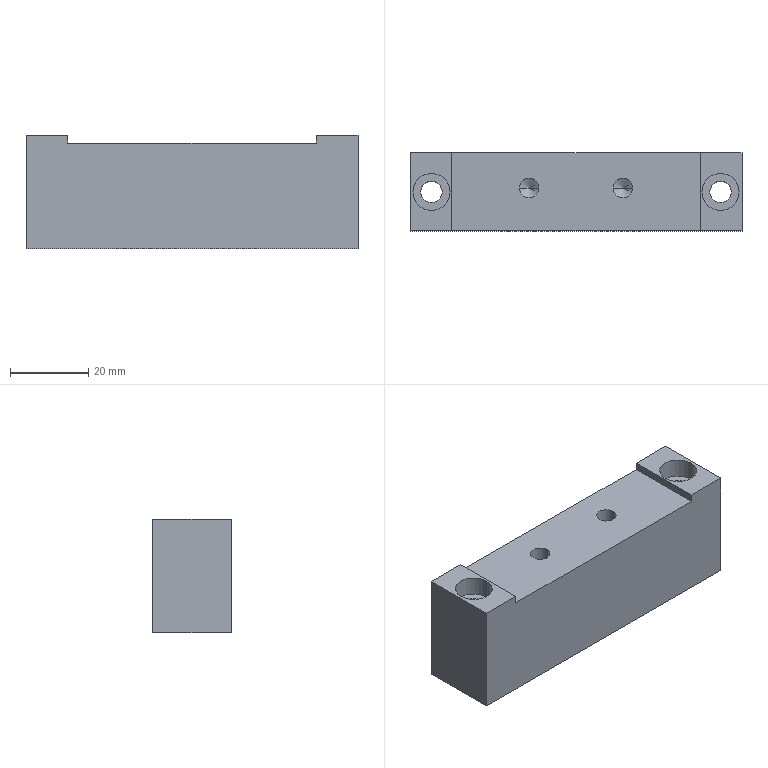Part | STEP file | 11-FG-E01211 | 1 solid | 28 faces | box 85 x 20 x 29 mm | volume 44302 mm3 | cylinder 12 | plane 12 | cone 4 | commonest cylinder face diameters 5 x4 5.5 x4 9.5 x4
STEP:
#1=CARTESIAN_POINT('',(-14.5,1.,12.));
#2=VERTEX_POINT('',#1);
#3=CARTESIAN_POINT('',(-9.5,1.,12.));
#4=VERTEX_POINT('',#3);
#5=CARTESIAN_POINT('',(-12.,1.,12.));
#6=DIRECTION('',(0.,0.,1.));
#7=DIRECTION('',(1.,0.,0.));
#8=AXIS2_PLACEMENT_3D('',#5,#6,#7);
#9=CIRCLE('',#8,2.5);
#10=EDGE_CURVE('',#2,#4,#9,.T.);
#11=ORIENTED_EDGE('',*,*,#10,.F.);
#12=CARTESIAN_POINT('',(-14.5,1.,27.));
#13=VERTEX_POINT('',#12);
#14=CARTESIAN_POINT('',(-14.5,1.,27.));
#15=DIRECTION('',(0.,0.,1.));
#16=VECTOR('',#15,1000.);
#17=LINE('',#14,#16);
#18=EDGE_CURVE('',#2,#13,#17,.T.);
#19=ORIENTED_EDGE('',*,*,#18,.T.);
#20=CARTESIAN_POINT('',(-9.5,1.,27.));
#21=VERTEX_POINT('',#20);
#22=CARTESIAN_POINT('',(-12.,1.,27.));
#23=DIRECTION('',(0.,0.,1.));
#24=DIRECTION('',(1.,0.,0.));
#25=AXIS2_PLACEMENT_3D('',#22,#23,#24);
#26=CIRCLE('',#25,2.5);
#27=EDGE_CURVE('',#13,#21,#26,.T.);
#28=ORIENTED_EDGE('',*,*,#27,.T.);
#29=CARTESIAN_POINT('',(-9.5,1.,27.));
#30=DIRECTION('',(0.,0.,1.));
#31=VECTOR('',#30,1000.);
#32=LINE('',#29,#31);
#33=EDGE_CURVE('',#4,#21,#32,.T.);
#34=ORIENTED_EDGE('',*,*,#33,.F.);
#35=EDGE_LOOP('',(#11,#19,#28,#34));
#36=FACE_OUTER_BOUND('',#35,.T.);
#37=CARTESIAN_POINT('',(-12.,1.,27.));
#38=DIRECTION('',(0.,0.,1.));
#39=DIRECTION('',(1.,0.,0.));
#40=AXIS2_PLACEMENT_3D('',#37,#38,#39);
#41=CYLINDRICAL_SURFACE('',#40,2.5);
#42=ADVANCED_FACE('',(#36),#41,.F.);
#43=CARTESIAN_POINT('',(-12.,1.,10.498));
#44=VERTEX_POINT('',#43);
#45=CARTESIAN_POINT('',(-9.5,1.,12.));
#46=DIRECTION('',(0.8572,0.,0.515));
#47=VECTOR('',#46,1000.);
#48=LINE('',#45,#47);
#49=EDGE_CURVE('',#44,#4,#48,.T.);
#50=ORIENTED_EDGE('',*,*,#49,.F.);
#51=CARTESIAN_POINT('',(-14.5,1.,12.));
#52=DIRECTION('',(-0.8572,0.,0.515));
#53=VECTOR('',#52,1000.);
#54=LINE('',#51,#53);
#55=EDGE_CURVE('',#44,#2,#54,.T.);
#56=ORIENTED_EDGE('',*,*,#55,.T.);
#57=ORIENTED_EDGE('',*,*,#10,.T.);
#58=EDGE_LOOP('',(#50,#56,#57));
#59=FACE_OUTER_BOUND('',#58,.T.);
#60=CARTESIAN_POINT('',(-12.,1.,12.));
#61=DIRECTION('',(0.,0.,1.));
#62=DIRECTION('',(1.,0.,0.));
#63=AXIS2_PLACEMENT_3D('',#60,#61,#62);
#64=CONICAL_SURFACE('',#63,2.5,1.03);
#65=ADVANCED_FACE('',(#59),#64,.F.);
#66=CARTESIAN_POINT('',(9.5,1.,12.));
#67=VERTEX_POINT('',#66);
#68=CARTESIAN_POINT('',(14.5,1.,12.));
#69=VERTEX_POINT('',#68);
#70=CARTESIAN_POINT('',(12.,1.,12.));
#71=DIRECTION('',(0.,0.,1.));
#72=DIRECTION('',(1.,0.,0.));
#73=AXIS2_PLACEMENT_3D('',#70,#71,#72);
#74=CIRCLE('',#73,2.5);
#75=EDGE_CURVE('',#67,#69,#74,.T.);
#76=ORIENTED_EDGE('',*,*,#75,.F.);
#77=CARTESIAN_POINT('',(9.5,1.,27.));
#78=VERTEX_POINT('',#77);
#79=CARTESIAN_POINT('',(9.5,1.,27.));
#80=DIRECTION('',(0.,0.,1.));
#81=VECTOR('',#80,1000.);
#82=LINE('',#79,#81);
#83=EDGE_CURVE('',#67,#78,#82,.T.);
#84=ORIENTED_EDGE('',*,*,#83,.T.);
#85=CARTESIAN_POINT('',(14.5,1.,27.));
#86=VERTEX_POINT('',#85);
#87=CARTESIAN_POINT('',(12.,1.,27.));
#88=DIRECTION('',(0.,0.,1.));
#89=DIRECTION('',(1.,0.,0.));
#90=AXIS2_PLACEMENT_3D('',#87,#88,#89);
#91=CIRCLE('',#90,2.5);
#92=EDGE_CURVE('',#78,#86,#91,.T.);
#93=ORIENTED_EDGE('',*,*,#92,.T.);
#94=CARTESIAN_POINT('',(14.5,1.,27.));
#95=DIRECTION('',(0.,0.,1.));
#96=VECTOR('',#95,1000.);
#97=LINE('',#94,#96);
#98=EDGE_CURVE('',#69,#86,#97,.T.);
#99=ORIENTED_EDGE('',*,*,#98,.F.);
#100=EDGE_LOOP('',(#76,#84,#93,#99));
#101=FACE_OUTER_BOUND('',#100,.T.);
#102=CARTESIAN_POINT('',(12.,1.,27.));
#103=DIRECTION('',(0.,0.,1.));
#104=DIRECTION('',(1.,0.,0.));
#105=AXIS2_PLACEMENT_3D('',#102,#103,#104);
#106=CYLINDRICAL_SURFACE('',#105,2.5);
#107=ADVANCED_FACE('',(#101),#106,.F.);
#108=CARTESIAN_POINT('',(12.,1.,10.498));
#109=VERTEX_POINT('',#108);
#110=CARTESIAN_POINT('',(14.5,1.,12.));
#111=DIRECTION('',(0.8572,0.,0.515));
#112=VECTOR('',#111,1000.);
#113=LINE('',#110,#112);
#114=EDGE_CURVE('',#109,#69,#113,.T.);
#115=ORIENTED_EDGE('',*,*,#114,.F.);
#116=CARTESIAN_POINT('',(9.5,1.,12.));
#117=DIRECTION('',(-0.8572,0.,0.515));
#118=VECTOR('',#117,1000.);
#119=LINE('',#116,#118);
#120=EDGE_CURVE('',#109,#67,#119,.T.);
#121=ORIENTED_EDGE('',*,*,#120,.T.);
#122=ORIENTED_EDGE('',*,*,#75,.T.);
#123=EDGE_LOOP('',(#115,#121,#122));
#124=FACE_OUTER_BOUND('',#123,.T.);
#125=CARTESIAN_POINT('',(12.,1.,12.));
#126=DIRECTION('',(0.,0.,1.));
#127=DIRECTION('',(1.,0.,0.));
#128=AXIS2_PLACEMENT_3D('',#125,#126,#127);
#129=CONICAL_SURFACE('',#128,2.5,1.03);
#130=ADVANCED_FACE('',(#124),#129,.F.);
#131=CARTESIAN_POINT('',(32.25,0.,24.));
#132=VERTEX_POINT('',#131);
#133=CARTESIAN_POINT('',(41.75,0.,24.));
#134=VERTEX_POINT('',#133);
#135=CARTESIAN_POINT('',(37.,0.,24.));
#136=DIRECTION('',(0.,0.,1.));
#137=DIRECTION('',(1.,0.,0.));
#138=AXIS2_PLACEMENT_3D('',#135,#136,#137);
#139=CIRCLE('',#138,4.75);
#140=EDGE_CURVE('',#132,#134,#139,.T.);
#141=ORIENTED_EDGE('',*,*,#140,.F.);
#142=CARTESIAN_POINT('',(32.25,0.,29.));
#143=VERTEX_POINT('',#142);
#144=CARTESIAN_POINT('',(32.25,0.,29.));
#145=DIRECTION('',(0.,0.,1.));
#146=VECTOR('',#145,1000.);
#147=LINE('',#144,#146);
#148=EDGE_CURVE('',#132,#143,#147,.T.);
#149=ORIENTED_EDGE('',*,*,#148,.T.);
#150=CARTESIAN_POINT('',(41.75,0.,29.));
#151=VERTEX_POINT('',#150);
#152=CARTESIAN_POINT('',(37.,0.,29.));
#153=DIRECTION('',(0.,0.,1.));
#154=DIRECTION('',(1.,0.,0.));
#155=AXIS2_PLACEMENT_3D('',#152,#153,#154);
#156=CIRCLE('',#155,4.75);
#157=EDGE_CURVE('',#143,#151,#156,.T.);
#158=ORIENTED_EDGE('',*,*,#157,.T.);
#159=CARTESIAN_POINT('',(41.75,0.,29.));
#160=DIRECTION('',(0.,0.,1.));
#161=VECTOR('',#160,1000.);
#162=LINE('',#159,#161);
#163=EDGE_CURVE('',#134,#151,#162,.T.);
#164=ORIENTED_EDGE('',*,*,#163,.F.);
#165=EDGE_LOOP('',(#141,#149,#158,#164));
#166=FACE_OUTER_BOUND('',#165,.T.);
#167=CARTESIAN_POINT('',(37.,0.,29.));
#168=DIRECTION('',(0.,0.,1.));
#169=DIRECTION('',(1.,0.,0.));
#170=AXIS2_PLACEMENT_3D('',#167,#168,#169);
#171=CYLINDRICAL_SURFACE('',#170,4.75);
#172=ADVANCED_FACE('',(#166),#171,.F.);
#173=CARTESIAN_POINT('',(34.25,0.,0.));
#174=VERTEX_POINT('',#173);
#175=CARTESIAN_POINT('',(39.75,0.,0.));
#176=VERTEX_POINT('',#175);
#177=CARTESIAN_POINT('',(37.,0.,0.));
#178=DIRECTION('',(0.,0.,1.));
#179=DIRECTION('',(1.,0.,0.));
#180=AXIS2_PLACEMENT_3D('',#177,#178,#179);
#181=CIRCLE('',#180,2.75);
#182=EDGE_CURVE('',#174,#176,#181,.T.);
#183=ORIENTED_EDGE('',*,*,#182,.F.);
#184=CARTESIAN_POINT('',(34.25,0.,24.));
#185=VERTEX_POINT('',#184);
#186=CARTESIAN_POINT('',(34.25,0.,29.));
#187=DIRECTION('',(0.,0.,1.));
#188=VECTOR('',#187,1000.);
#189=LINE('',#186,#188);
#190=EDGE_CURVE('',#174,#185,#189,.T.);
#191=ORIENTED_EDGE('',*,*,#190,.T.);
#192=CARTESIAN_POINT('',(39.75,0.,24.));
#193=VERTEX_POINT('',#192);
#194=CARTESIAN_POINT('',(37.,0.,24.));
#195=DIRECTION('',(0.,0.,1.));
#196=DIRECTION('',(1.,0.,0.));
#197=AXIS2_PLACEMENT_3D('',#194,#195,#196);
#198=CIRCLE('',#197,2.75);
#199=EDGE_CURVE('',#185,#193,#198,.T.);
#200=ORIENTED_EDGE('',*,*,#199,.T.);
#201=CARTESIAN_POINT('',(39.75,0.,29.));
#202=DIRECTION('',(0.,0.,1.));
#203=VECTOR('',#202,1000.);
#204=LINE('',#201,#203);
#205=EDGE_CURVE('',#176,#193,#204,.T.);
#206=ORIENTED_EDGE('',*,*,#205,.F.);
#207=EDGE_LOOP('',(#183,#191,#200,#206));
#208=FACE_OUTER_BOUND('',#207,.T.);
#209=CARTESIAN_POINT('',(37.,0.,29.));
#210=DIRECTION('',(0.,0.,1.));
#211=DIRECTION('',(1.,0.,0.));
#212=AXIS2_PLACEMENT_3D('',#209,#210,#211);
#213=CYLINDRICAL_SURFACE('',#212,2.75);
#214=ADVANCED_FACE('',(#208),#213,.F.);
#215=CARTESIAN_POINT('',(-41.75,0.,24.));
#216=VERTEX_POINT('',#215);
#217=CARTESIAN_POINT('',(-32.25,0.,24.));
#218=VERTEX_POINT('',#217);
#219=CARTESIAN_POINT('',(-37.,0.,24.));
#220=DIRECTION('',(0.,0.,1.));
#221=DIRECTION('',(1.,0.,0.));
#222=AXIS2_PLACEMENT_3D('',#219,#220,#221);
#223=CIRCLE('',#222,4.75);
#224=EDGE_CURVE('',#216,#218,#223,.T.);
#225=ORIENTED_EDGE('',*,*,#224,.F.);
#226=CARTESIAN_POINT('',(-41.75,0.,29.));
#227=VERTEX_POINT('',#226);
#228=CARTESIAN_POINT('',(-41.75,0.,29.));
#229=DIRECTION('',(0.,0.,1.));
#230=VECTOR('',#229,1000.);
#231=LINE('',#228,#230);
#232=EDGE_CURVE('',#216,#227,#231,.T.);
#233=ORIENTED_EDGE('',*,*,#232,.T.);
#234=CARTESIAN_POINT('',(-32.25,0.,29.));
#235=VERTEX_POINT('',#234);
#236=CARTESIAN_POINT('',(-37.,0.,29.));
#237=DIRECTION('',(0.,0.,1.));
#238=DIRECTION('',(1.,0.,0.));
#239=AXIS2_PLACEMENT_3D('',#236,#237,#238);
#240=CIRCLE('',#239,4.75);
#241=EDGE_CURVE('',#227,#235,#240,.T.);
#242=ORIENTED_EDGE('',*,*,#241,.T.);
#243=CARTESIAN_POINT('',(-32.25,0.,29.));
#244=DIRECTION('',(0.,0.,1.));
#245=VECTOR('',#244,1000.);
#246=LINE('',#243,#245);
#247=EDGE_CURVE('',#218,#235,#246,.T.);
#248=ORIENTED_EDGE('',*,*,#247,.F.);
#249=EDGE_LOOP('',(#225,#233,#242,#248));
#250=FACE_OUTER_BOUND('',#249,.T.);
#251=CARTESIAN_POINT('',(-37.,0.,29.));
#252=DIRECTION('',(0.,0.,1.));
#253=DIRECTION('',(1.,0.,0.));
#254=AXIS2_PLACEMENT_3D('',#251,#252,#253);
#255=CYLINDRICAL_SURFACE('',#254,4.75);
#256=ADVANCED_FACE('',(#250),#255,.F.);
#257=CARTESIAN_POINT('',(-39.75,0.,0.));
#258=VERTEX_POINT('',#257);
#259=CARTESIAN_POINT('',(-34.25,0.,0.));
#260=VERTEX_POINT('',#259);
#261=CARTESIAN_POINT('',(-37.,0.,0.));
#262=DIRECTION('',(0.,0.,1.));
#263=DIRECTION('',(1.,0.,0.));
#264=AXIS2_PLACEMENT_3D('',#261,#262,#263);
#265=CIRCLE('',#264,2.75);
#266=EDGE_CURVE('',#258,#260,#265,.T.);
#267=ORIENTED_EDGE('',*,*,#266,.F.);
#268=CARTESIAN_POINT('',(-39.75,0.,24.));
#269=VERTEX_POINT('',#268);
#270=CARTESIAN_POINT('',(-39.75,0.,29.));
#271=DIRECTION('',(0.,0.,1.));
#272=VECTOR('',#271,1000.);
#273=LINE('',#270,#272);
#274=EDGE_CURVE('',#258,#269,#273,.T.);
#275=ORIENTED_EDGE('',*,*,#274,.T.);
#276=CARTESIAN_POINT('',(-34.25,0.,24.));
#277=VERTEX_POINT('',#276);
#278=CARTESIAN_POINT('',(-37.,0.,24.));
#279=DIRECTION('',(0.,0.,1.));
#280=DIRECTION('',(1.,0.,0.));
#281=AXIS2_PLACEMENT_3D('',#278,#279,#280);
#282=CIRCLE('',#281,2.75);
#283=EDGE_CURVE('',#269,#277,#282,.T.);
#284=ORIENTED_EDGE('',*,*,#283,.T.);
#285=CARTESIAN_POINT('',(-34.25,0.,29.));
#286=DIRECTION('',(0.,0.,1.));
#287=VECTOR('',#286,1000.);
#288=LINE('',#285,#287);
#289=EDGE_CURVE('',#260,#277,#288,.T.);
#290=ORIENTED_EDGE('',*,*,#289,.F.);
#291=EDGE_LOOP('',(#267,#275,#284,#290));
#292=FACE_OUTER_BOUND('',#291,.T.);
#293=CARTESIAN_POINT('',(-37.,0.,29.));
#294=DIRECTION('',(0.,0.,1.));
#295=DIRECTION('',(1.,0.,0.));
#296=AXIS2_PLACEMENT_3D('',#293,#294,#295);
#297=CYLINDRICAL_SURFACE('',#296,2.75);
#298=ADVANCED_FACE('',(#292),#297,.F.);
#299=CARTESIAN_POINT('',(-37.,0.,29.));
#300=DIRECTION('',(0.,0.,1.));
#301=DIRECTION('',(1.,0.,0.));
#302=AXIS2_PLACEMENT_3D('',#299,#300,#301);
#303=CIRCLE('',#302,4.75);
#304=EDGE_CURVE('',#235,#227,#303,.T.);
#305=ORIENTED_EDGE('',*,*,#304,.F.);
#306=ORIENTED_EDGE('',*,*,#241,.F.);
#307=EDGE_LOOP('',(#305,#306));
#308=FACE_BOUND('',#307,.T.);
#309=CARTESIAN_POINT('',(-31.75,-10.,29.));
#310=VERTEX_POINT('',#309);
#311=CARTESIAN_POINT('',(-31.75,10.,29.));
#312=VERTEX_POINT('',#311);
#313=CARTESIAN_POINT('',(-31.75,-10.,29.));
#314=DIRECTION('',(0.,1.,0.));
#315=VECTOR('',#314,1000.);
#316=LINE('',#313,#315);
#317=EDGE_CURVE('',#310,#312,#316,.T.);
#318=ORIENTED_EDGE('',*,*,#317,.T.);
#319=CARTESIAN_POINT('',(-42.5,10.,29.));
#320=VERTEX_POINT('',#319);
#321=CARTESIAN_POINT('',(-42.5,10.,29.));
#322=DIRECTION('',(-1.,0.,0.));
#323=VECTOR('',#322,1000.);
#324=LINE('',#321,#323);
#325=EDGE_CURVE('',#312,#320,#324,.T.);
#326=ORIENTED_EDGE('',*,*,#325,.T.);
#327=CARTESIAN_POINT('',(-42.5,-10.,29.));
#328=VERTEX_POINT('',#327);
#329=CARTESIAN_POINT('',(-42.5,10.,29.));
#330=DIRECTION('',(0.,-1.,0.));
#331=VECTOR('',#330,1000.);
#332=LINE('',#329,#331);
#333=EDGE_CURVE('',#320,#328,#332,.T.);
#334=ORIENTED_EDGE('',*,*,#333,.T.);
#335=CARTESIAN_POINT('',(-42.5,-10.,29.));
#336=DIRECTION('',(1.,0.,0.));
#337=VECTOR('',#336,1000.);
#338=LINE('',#335,#337);
#339=EDGE_CURVE('',#328,#310,#338,.T.);
#340=ORIENTED_EDGE('',*,*,#339,.T.);
#341=EDGE_LOOP('',(#318,#326,#334,#340));
#342=FACE_OUTER_BOUND('',#341,.T.);
#343=CARTESIAN_POINT('',(42.5,-10.,29.));
#344=DIRECTION('',(0.,0.,1.));
#345=DIRECTION('',(1.,0.,0.));
#346=AXIS2_PLACEMENT_3D('',#343,#344,#345);
#347=PLANE('',#346);
#348=ADVANCED_FACE('',(#308,#342),#347,.T.);
#349=CARTESIAN_POINT('',(42.5,-10.,0.));
#350=VERTEX_POINT('',#349);
#351=CARTESIAN_POINT('',(42.5,10.,0.));
#352=VERTEX_POINT('',#351);
#353=CARTESIAN_POINT('',(42.5,10.,0.));
#354=DIRECTION('',(0.,1.,0.));
#355=VECTOR('',#354,1000.);
#356=LINE('',#353,#355);
#357=EDGE_CURVE('',#350,#352,#356,.T.);
#358=ORIENTED_EDGE('',*,*,#357,.T.);
#359=CARTESIAN_POINT('',(42.5,10.,29.));
#360=VERTEX_POINT('',#359);
#361=CARTESIAN_POINT('',(42.5,10.,29.));
#362=DIRECTION('',(0.,0.,-1.));
#363=VECTOR('',#362,1000.);
#364=LINE('',#361,#363);
#365=EDGE_CURVE('',#360,#352,#364,.T.);
#366=ORIENTED_EDGE('',*,*,#365,.F.);
#367=CARTESIAN_POINT('',(42.5,-10.,29.));
#368=VERTEX_POINT('',#367);
#369=CARTESIAN_POINT('',(42.5,10.,29.));
#370=DIRECTION('',(0.,1.,0.));
#371=VECTOR('',#370,1000.);
#372=LINE('',#369,#371);
#373=EDGE_CURVE('',#368,#360,#372,.T.);
#374=ORIENTED_EDGE('',*,*,#373,.F.);
#375=CARTESIAN_POINT('',(42.5,-10.,29.));
#376=DIRECTION('',(0.,0.,-1.));
#377=VECTOR('',#376,1000.);
#378=LINE('',#375,#377);
#379=EDGE_CURVE('',#368,#350,#378,.T.);
#380=ORIENTED_EDGE('',*,*,#379,.T.);
#381=EDGE_LOOP('',(#358,#366,#374,#380));
#382=FACE_OUTER_BOUND('',#381,.T.);
#383=CARTESIAN_POINT('',(42.5,10.,29.));
#384=DIRECTION('',(-1.,0.,0.));
#385=DIRECTION('',(0.,0.,1.));
#386=AXIS2_PLACEMENT_3D('',#383,#384,#385);
#387=PLANE('',#386);
#388=ADVANCED_FACE('',(#382),#387,.F.);
#389=ORIENTED_EDGE('',*,*,#325,.F.);
#390=CARTESIAN_POINT('',(-31.75,10.,27.));
#391=VERTEX_POINT('',#390);
#392=CARTESIAN_POINT('',(-31.75,10.,27.));
#393=DIRECTION('',(0.,0.,1.));
#394=VECTOR('',#393,1000.);
#395=LINE('',#392,#394);
#396=EDGE_CURVE('',#391,#312,#395,.T.);
#397=ORIENTED_EDGE('',*,*,#396,.F.);
#398=CARTESIAN_POINT('',(31.75,10.,27.));
#399=VERTEX_POINT('',#398);
#400=CARTESIAN_POINT('',(-31.75,10.,27.));
#401=DIRECTION('',(-1.,0.,0.));
#402=VECTOR('',#401,1000.);
#403=LINE('',#400,#402);
#404=EDGE_CURVE('',#399,#391,#403,.T.);
#405=ORIENTED_EDGE('',*,*,#404,.F.);
#406=CARTESIAN_POINT('',(31.75,10.,29.));
#407=VERTEX_POINT('',#406);
#408=CARTESIAN_POINT('',(31.75,10.,27.));
#409=DIRECTION('',(0.,0.,-1.));
#410=VECTOR('',#409,1000.);
#411=LINE('',#408,#410);
#412=EDGE_CURVE('',#407,#399,#411,.T.);
#413=ORIENTED_EDGE('',*,*,#412,.F.);
#414=CARTESIAN_POINT('',(-42.5,10.,29.));
#415=DIRECTION('',(-1.,0.,0.));
#416=VECTOR('',#415,1000.);
#417=LINE('',#414,#416);
#418=EDGE_CURVE('',#360,#407,#417,.T.);
#419=ORIENTED_EDGE('',*,*,#418,.F.);
#420=ORIENTED_EDGE('',*,*,#365,.T.);
#421=CARTESIAN_POINT('',(-42.5,10.,0.));
#422=VERTEX_POINT('',#421);
#423=CARTESIAN_POINT('',(-42.5,10.,0.));
#424=DIRECTION('',(-1.,0.,0.));
#425=VECTOR('',#424,1000.);
#426=LINE('',#423,#425);
#427=EDGE_CURVE('',#352,#422,#426,.T.);
#428=ORIENTED_EDGE('',*,*,#427,.T.);
#429=CARTESIAN_POINT('',(-42.5,10.,29.));
#430=DIRECTION('',(0.,0.,-1.));
#431=VECTOR('',#430,1000.);
#432=LINE('',#429,#431);
#433=EDGE_CURVE('',#320,#422,#432,.T.);
#434=ORIENTED_EDGE('',*,*,#433,.F.);
#435=EDGE_LOOP('',(#389,#397,#405,#413,#419,#420,#428,#434));
#436=FACE_OUTER_BOUND('',#435,.T.);
#437=CARTESIAN_POINT('',(-42.5,10.,29.));
#438=DIRECTION('',(0.,-1.,0.));
#439=DIRECTION('',(0.,0.,-1.));
#440=AXIS2_PLACEMENT_3D('',#437,#438,#439);
#441=PLANE('',#440);
#442=ADVANCED_FACE('',(#436),#441,.F.);
#443=CARTESIAN_POINT('',(-42.5,-10.,0.));
#444=VERTEX_POINT('',#443);
#445=CARTESIAN_POINT('',(-42.5,10.,0.));
#446=DIRECTION('',(0.,-1.,0.));
#447=VECTOR('',#446,1000.);
#448=LINE('',#445,#447);
#449=EDGE_CURVE('',#422,#444,#448,.T.);
#450=ORIENTED_EDGE('',*,*,#449,.T.);
#451=CARTESIAN_POINT('',(-42.5,-10.,29.));
#452=DIRECTION('',(0.,0.,-1.));
#453=VECTOR('',#452,1000.);
#454=LINE('',#451,#453);
#455=EDGE_CURVE('',#328,#444,#454,.T.);
#456=ORIENTED_EDGE('',*,*,#455,.F.);
#457=ORIENTED_EDGE('',*,*,#333,.F.);
#458=ORIENTED_EDGE('',*,*,#433,.T.);
#459=EDGE_LOOP('',(#450,#456,#457,#458));
#460=FACE_OUTER_BOUND('',#459,.T.);
#461=CARTESIAN_POINT('',(-42.5,10.,29.));
#462=DIRECTION('',(1.,0.,0.));
#463=DIRECTION('',(0.,0.,-1.));
#464=AXIS2_PLACEMENT_3D('',#461,#462,#463);
#465=PLANE('',#464);
#466=ADVANCED_FACE('',(#460),#465,.F.);
#467=CARTESIAN_POINT('',(31.75,-10.,27.));
#468=VERTEX_POINT('',#467);
#469=CARTESIAN_POINT('',(-31.75,-10.,27.));
#470=VERTEX_POINT('',#469);
#471=CARTESIAN_POINT('',(-31.75,-10.,27.));
#472=DIRECTION('',(-1.,0.,0.));
#473=VECTOR('',#472,1000.);
#474=LINE('',#471,#473);
#475=EDGE_CURVE('',#468,#470,#474,.T.);
#476=ORIENTED_EDGE('',*,*,#475,.T.);
#477=CARTESIAN_POINT('',(-31.75,-10.,27.));
#478=DIRECTION('',(0.,0.,1.));
#479=VECTOR('',#478,1000.);
#480=LINE('',#477,#479);
#481=EDGE_CURVE('',#470,#310,#480,.T.);
#482=ORIENTED_EDGE('',*,*,#481,.T.);
#483=ORIENTED_EDGE('',*,*,#339,.F.);
#484=ORIENTED_EDGE('',*,*,#455,.T.);
#485=CARTESIAN_POINT('',(-42.5,-10.,0.));
#486=DIRECTION('',(1.,0.,0.));
#487=VECTOR('',#486,1000.);
#488=LINE('',#485,#487);
#489=EDGE_CURVE('',#444,#350,#488,.T.);
#490=ORIENTED_EDGE('',*,*,#489,.T.);
#491=ORIENTED_EDGE('',*,*,#379,.F.);
#492=CARTESIAN_POINT('',(31.75,-10.,29.));
#493=VERTEX_POINT('',#492);
#494=CARTESIAN_POINT('',(-42.5,-10.,29.));
#495=DIRECTION('',(1.,0.,0.));
#496=VECTOR('',#495,1000.);
#497=LINE('',#494,#496);
#498=EDGE_CURVE('',#493,#368,#497,.T.);
#499=ORIENTED_EDGE('',*,*,#498,.F.);
#500=CARTESIAN_POINT('',(31.75,-10.,27.));
#501=DIRECTION('',(0.,0.,-1.));
#502=VECTOR('',#501,1000.);
#503=LINE('',#500,#502);
#504=EDGE_CURVE('',#493,#468,#503,.T.);
#505=ORIENTED_EDGE('',*,*,#504,.T.);
#506=EDGE_LOOP('',(#476,#482,#483,#484,#490,#491,#499,#505));
#507=FACE_OUTER_BOUND('',#506,.T.);
#508=CARTESIAN_POINT('',(-42.5,-10.,29.));
#509=DIRECTION('',(0.,1.,0.));
#510=DIRECTION('',(0.,0.,1.));
#511=AXIS2_PLACEMENT_3D('',#508,#509,#510);
#512=PLANE('',#511);
#513=ADVANCED_FACE('',(#507),#512,.F.);
#514=CARTESIAN_POINT('',(37.,0.,29.));
#515=DIRECTION('',(0.,0.,1.));
#516=DIRECTION('',(1.,0.,0.));
#517=AXIS2_PLACEMENT_3D('',#514,#515,#516);
#518=CIRCLE('',#517,4.75);
#519=EDGE_CURVE('',#151,#143,#518,.T.);
#520=ORIENTED_EDGE('',*,*,#519,.F.);
#521=ORIENTED_EDGE('',*,*,#157,.F.);
#522=EDGE_LOOP('',(#520,#521));
#523=FACE_BOUND('',#522,.T.);
#524=CARTESIAN_POINT('',(31.75,-10.,29.));
#525=DIRECTION('',(0.,1.,0.));
#526=VECTOR('',#525,1000.);
#527=LINE('',#524,#526);
#528=EDGE_CURVE('',#493,#407,#527,.T.);
#529=ORIENTED_EDGE('',*,*,#528,.F.);
#530=ORIENTED_EDGE('',*,*,#498,.T.);
#531=ORIENTED_EDGE('',*,*,#373,.T.);
#532=ORIENTED_EDGE('',*,*,#418,.T.);
#533=EDGE_LOOP('',(#529,#530,#531,#532));
#534=FACE_OUTER_BOUND('',#533,.T.);
#535=CARTESIAN_POINT('',(42.5,-10.,29.));
#536=DIRECTION('',(0.,0.,1.));
#537=DIRECTION('',(1.,0.,0.));
#538=AXIS2_PLACEMENT_3D('',#535,#536,#537);
#539=PLANE('',#538);
#540=ADVANCED_FACE('',(#523,#534),#539,.T.);
#541=CARTESIAN_POINT('',(37.,0.,0.));
#542=DIRECTION('',(0.,0.,1.));
#543=DIRECTION('',(1.,0.,0.));
#544=AXIS2_PLACEMENT_3D('',#541,#542,#543);
#545=CIRCLE('',#544,2.75);
#546=EDGE_CURVE('',#176,#174,#545,.T.);
#547=ORIENTED_EDGE('',*,*,#546,.T.);
#548=ORIENTED_EDGE('',*,*,#182,.T.);
#549=EDGE_LOOP('',(#547,#548));
#550=FACE_BOUND('',#549,.T.);
#551=CARTESIAN_POINT('',(-37.,0.,0.));
#552=DIRECTION('',(0.,0.,1.));
#553=DIRECTION('',(1.,0.,0.));
#554=AXIS2_PLACEMENT_3D('',#551,#552,#553);
#555=CIRCLE('',#554,2.75);
#556=EDGE_CURVE('',#260,#258,#555,.T.);
#557=ORIENTED_EDGE('',*,*,#556,.T.);
#558=ORIENTED_EDGE('',*,*,#266,.T.);
#559=EDGE_LOOP('',(#557,#558));
#560=FACE_BOUND('',#559,.T.);
#561=ORIENTED_EDGE('',*,*,#357,.F.);
#562=ORIENTED_EDGE('',*,*,#489,.F.);
#563=ORIENTED_EDGE('',*,*,#449,.F.);
#564=ORIENTED_EDGE('',*,*,#427,.F.);
#565=EDGE_LOOP('',(#561,#562,#563,#564));
#566=FACE_OUTER_BOUND('',#565,.T.);
#567=CARTESIAN_POINT('',(42.5,-10.,0.));
#568=DIRECTION('',(0.,0.,1.));
#569=DIRECTION('',(1.,0.,0.));
#570=AXIS2_PLACEMENT_3D('',#567,#568,#569);
#571=PLANE('',#570);
#572=ADVANCED_FACE('',(#550,#560,#566),#571,.F.);
#573=ORIENTED_EDGE('',*,*,#396,.T.);
#574=ORIENTED_EDGE('',*,*,#317,.F.);
#575=ORIENTED_EDGE('',*,*,#481,.F.);
#576=CARTESIAN_POINT('',(-31.75,-10.,27.));
#577=DIRECTION('',(0.,1.,0.));
#578=VECTOR('',#577,1000.);
#579=LINE('',#576,#578);
#580=EDGE_CURVE('',#470,#391,#579,.T.);
#581=ORIENTED_EDGE('',*,*,#580,.T.);
#582=EDGE_LOOP('',(#573,#574,#575,#581));
#583=FACE_OUTER_BOUND('',#582,.T.);
#584=CARTESIAN_POINT('',(-31.75,-10.,27.));
#585=DIRECTION('',(-1.,0.,0.));
#586=DIRECTION('',(0.,0.,1.));
#587=AXIS2_PLACEMENT_3D('',#584,#585,#586);
#588=PLANE('',#587);
#589=ADVANCED_FACE('',(#583),#588,.F.);
#590=CARTESIAN_POINT('',(-12.,1.,27.));
#591=DIRECTION('',(0.,0.,1.));
#592=DIRECTION('',(1.,0.,0.));
#593=AXIS2_PLACEMENT_3D('',#590,#591,#592);
#594=CIRCLE('',#593,2.5);
#595=EDGE_CURVE('',#21,#13,#594,.T.);
#596=ORIENTED_EDGE('',*,*,#595,.F.);
#597=ORIENTED_EDGE('',*,*,#27,.F.);
#598=EDGE_LOOP('',(#596,#597));
#599=FACE_BOUND('',#598,.T.);
#600=CARTESIAN_POINT('',(12.,1.,27.));
#601=DIRECTION('',(0.,0.,1.));
#602=DIRECTION('',(1.,0.,0.));
#603=AXIS2_PLACEMENT_3D('',#600,#601,#602);
#604=CIRCLE('',#603,2.5);
#605=EDGE_CURVE('',#86,#78,#604,.T.);
#606=ORIENTED_EDGE('',*,*,#605,.F.);
#607=ORIENTED_EDGE('',*,*,#92,.F.);
#608=EDGE_LOOP('',(#606,#607));
#609=FACE_BOUND('',#608,.T.);
#610=ORIENTED_EDGE('',*,*,#404,.T.);
#611=ORIENTED_EDGE('',*,*,#580,.F.);
#612=ORIENTED_EDGE('',*,*,#475,.F.);
#613=CARTESIAN_POINT('',(31.75,-10.,27.));
#614=DIRECTION('',(0.,1.,0.));
#615=VECTOR('',#614,1000.);
#616=LINE('',#613,#615);
#617=EDGE_CURVE('',#468,#399,#616,.T.);
#618=ORIENTED_EDGE('',*,*,#617,.T.);
#619=EDGE_LOOP('',(#610,#611,#612,#618));
#620=FACE_OUTER_BOUND('',#619,.T.);
#621=CARTESIAN_POINT('',(-31.75,-10.,27.));
#622=DIRECTION('',(0.,0.,-1.));
#623=DIRECTION('',(-1.,0.,0.));
#624=AXIS2_PLACEMENT_3D('',#621,#622,#623);
#625=PLANE('',#624);
#626=ADVANCED_FACE('',(#599,#609,#620),#625,.F.);
#627=ORIENTED_EDGE('',*,*,#412,.T.);
#628=ORIENTED_EDGE('',*,*,#617,.F.);
#629=ORIENTED_EDGE('',*,*,#504,.F.);
#630=ORIENTED_EDGE('',*,*,#528,.T.);
#631=EDGE_LOOP('',(#627,#628,#629,#630));
#632=FACE_OUTER_BOUND('',#631,.T.);
#633=CARTESIAN_POINT('',(31.75,-10.,27.));
#634=DIRECTION('',(1.,0.,0.));
#635=DIRECTION('',(0.,0.,-1.));
#636=AXIS2_PLACEMENT_3D('',#633,#634,#635);
#637=PLANE('',#636);
#638=ADVANCED_FACE('',(#632),#637,.F.);
#639=ORIENTED_EDGE('',*,*,#274,.F.);
#640=ORIENTED_EDGE('',*,*,#556,.F.);
#641=ORIENTED_EDGE('',*,*,#289,.T.);
#642=CARTESIAN_POINT('',(-37.,0.,24.));
#643=DIRECTION('',(0.,0.,1.));
#644=DIRECTION('',(1.,0.,0.));
#645=AXIS2_PLACEMENT_3D('',#642,#643,#644);
#646=CIRCLE('',#645,2.75);
#647=EDGE_CURVE('',#277,#269,#646,.T.);
#648=ORIENTED_EDGE('',*,*,#647,.T.);
#649=EDGE_LOOP('',(#639,#640,#641,#648));
#650=FACE_OUTER_BOUND('',#649,.T.);
#651=CARTESIAN_POINT('',(-37.,0.,29.));
#652=DIRECTION('',(0.,0.,1.));
#653=DIRECTION('',(1.,0.,0.));
#654=AXIS2_PLACEMENT_3D('',#651,#652,#653);
#655=CYLINDRICAL_SURFACE('',#654,2.75);
#656=ADVANCED_FACE('',(#650),#655,.F.);
#657=ORIENTED_EDGE('',*,*,#647,.F.);
#658=ORIENTED_EDGE('',*,*,#283,.F.);
#659=EDGE_LOOP('',(#657,#658));
#660=FACE_BOUND('',#659,.T.);
#661=CARTESIAN_POINT('',(-37.,0.,24.));
#662=DIRECTION('',(0.,0.,1.));
#663=DIRECTION('',(1.,0.,0.));
#664=AXIS2_PLACEMENT_3D('',#661,#662,#663);
#665=CIRCLE('',#664,4.75);
#666=EDGE_CURVE('',#218,#216,#665,.T.);
#667=ORIENTED_EDGE('',*,*,#666,.T.);
#668=ORIENTED_EDGE('',*,*,#224,.T.);
#669=EDGE_LOOP('',(#667,#668));
#670=FACE_OUTER_BOUND('',#669,.T.);
#671=CARTESIAN_POINT('',(-34.25,0.,24.));
#672=DIRECTION('',(0.,0.,-1.));
#673=DIRECTION('',(-1.,0.,0.));
#674=AXIS2_PLACEMENT_3D('',#671,#672,#673);
#675=PLANE('',#674);
#676=ADVANCED_FACE('',(#660,#670),#675,.F.);
#677=ORIENTED_EDGE('',*,*,#232,.F.);
#678=ORIENTED_EDGE('',*,*,#666,.F.);
#679=ORIENTED_EDGE('',*,*,#247,.T.);
#680=ORIENTED_EDGE('',*,*,#304,.T.);
#681=EDGE_LOOP('',(#677,#678,#679,#680));
#682=FACE_OUTER_BOUND('',#681,.T.);
#683=CARTESIAN_POINT('',(-37.,0.,29.));
#684=DIRECTION('',(0.,0.,1.));
#685=DIRECTION('',(1.,0.,0.));
#686=AXIS2_PLACEMENT_3D('',#683,#684,#685);
#687=CYLINDRICAL_SURFACE('',#686,4.75);
#688=ADVANCED_FACE('',(#682),#687,.F.);
#689=ORIENTED_EDGE('',*,*,#190,.F.);
#690=ORIENTED_EDGE('',*,*,#546,.F.);
#691=ORIENTED_EDGE('',*,*,#205,.T.);
#692=CARTESIAN_POINT('',(37.,0.,24.));
#693=DIRECTION('',(0.,0.,1.));
#694=DIRECTION('',(1.,0.,0.));
#695=AXIS2_PLACEMENT_3D('',#692,#693,#694);
#696=CIRCLE('',#695,2.75);
#697=EDGE_CURVE('',#193,#185,#696,.T.);
#698=ORIENTED_EDGE('',*,*,#697,.T.);
#699=EDGE_LOOP('',(#689,#690,#691,#698));
#700=FACE_OUTER_BOUND('',#699,.T.);
#701=CARTESIAN_POINT('',(37.,0.,29.));
#702=DIRECTION('',(0.,0.,1.));
#703=DIRECTION('',(1.,0.,0.));
#704=AXIS2_PLACEMENT_3D('',#701,#702,#703);
#705=CYLINDRICAL_SURFACE('',#704,2.75);
#706=ADVANCED_FACE('',(#700),#705,.F.);
#707=ORIENTED_EDGE('',*,*,#697,.F.);
#708=ORIENTED_EDGE('',*,*,#199,.F.);
#709=EDGE_LOOP('',(#707,#708));
#710=FACE_BOUND('',#709,.T.);
#711=CARTESIAN_POINT('',(37.,0.,24.));
#712=DIRECTION('',(0.,0.,1.));
#713=DIRECTION('',(1.,0.,0.));
#714=AXIS2_PLACEMENT_3D('',#711,#712,#713);
#715=CIRCLE('',#714,4.75);
#716=EDGE_CURVE('',#134,#132,#715,.T.);
#717=ORIENTED_EDGE('',*,*,#716,.T.);
#718=ORIENTED_EDGE('',*,*,#140,.T.);
#719=EDGE_LOOP('',(#717,#718));
#720=FACE_OUTER_BOUND('',#719,.T.);
#721=CARTESIAN_POINT('',(39.75,0.,24.));
#722=DIRECTION('',(0.,0.,-1.));
#723=DIRECTION('',(-1.,0.,0.));
#724=AXIS2_PLACEMENT_3D('',#721,#722,#723);
#725=PLANE('',#724);
#726=ADVANCED_FACE('',(#710,#720),#725,.F.);
#727=ORIENTED_EDGE('',*,*,#148,.F.);
#728=ORIENTED_EDGE('',*,*,#716,.F.);
#729=ORIENTED_EDGE('',*,*,#163,.T.);
#730=ORIENTED_EDGE('',*,*,#519,.T.);
#731=EDGE_LOOP('',(#727,#728,#729,#730));
#732=FACE_OUTER_BOUND('',#731,.T.);
#733=CARTESIAN_POINT('',(37.,0.,29.));
#734=DIRECTION('',(0.,0.,1.));
#735=DIRECTION('',(1.,0.,0.));
#736=AXIS2_PLACEMENT_3D('',#733,#734,#735);
#737=CYLINDRICAL_SURFACE('',#736,4.75);
#738=ADVANCED_FACE('',(#732),#737,.F.);
#739=ORIENTED_EDGE('',*,*,#120,.F.);
#740=ORIENTED_EDGE('',*,*,#114,.T.);
#741=CARTESIAN_POINT('',(12.,1.,12.));
#742=DIRECTION('',(0.,0.,1.));
#743=DIRECTION('',(1.,0.,0.));
#744=AXIS2_PLACEMENT_3D('',#741,#742,#743);
#745=CIRCLE('',#744,2.5);
#746=EDGE_CURVE('',#69,#67,#745,.T.);
#747=ORIENTED_EDGE('',*,*,#746,.T.);
#748=EDGE_LOOP('',(#739,#740,#747));
#749=FACE_OUTER_BOUND('',#748,.T.);
#750=CARTESIAN_POINT('',(12.,1.,12.));
#751=DIRECTION('',(0.,0.,1.));
#752=DIRECTION('',(1.,0.,0.));
#753=AXIS2_PLACEMENT_3D('',#750,#751,#752);
#754=CONICAL_SURFACE('',#753,2.5,1.03);
#755=ADVANCED_FACE('',(#749),#754,.F.);
#756=ORIENTED_EDGE('',*,*,#83,.F.);
#757=ORIENTED_EDGE('',*,*,#746,.F.);
#758=ORIENTED_EDGE('',*,*,#98,.T.);
#759=ORIENTED_EDGE('',*,*,#605,.T.);
#760=EDGE_LOOP('',(#756,#757,#758,#759));
#761=FACE_OUTER_BOUND('',#760,.T.);
#762=CARTESIAN_POINT('',(12.,1.,27.));
#763=DIRECTION('',(0.,0.,1.));
#764=DIRECTION('',(1.,0.,0.));
#765=AXIS2_PLACEMENT_3D('',#762,#763,#764);
#766=CYLINDRICAL_SURFACE('',#765,2.5);
#767=ADVANCED_FACE('',(#761),#766,.F.);
#768=ORIENTED_EDGE('',*,*,#55,.F.);
#769=ORIENTED_EDGE('',*,*,#49,.T.);
#770=CARTESIAN_POINT('',(-12.,1.,12.));
#771=DIRECTION('',(0.,0.,1.));
#772=DIRECTION('',(1.,0.,0.));
#773=AXIS2_PLACEMENT_3D('',#770,#771,#772);
#774=CIRCLE('',#773,2.5);
#775=EDGE_CURVE('',#4,#2,#774,.T.);
#776=ORIENTED_EDGE('',*,*,#775,.T.);
#777=EDGE_LOOP('',(#768,#769,#776));
#778=FACE_OUTER_BOUND('',#777,.T.);
#779=CARTESIAN_POINT('',(-12.,1.,12.));
#780=DIRECTION('',(0.,0.,1.));
#781=DIRECTION('',(1.,0.,0.));
#782=AXIS2_PLACEMENT_3D('',#779,#780,#781);
#783=CONICAL_SURFACE('',#782,2.5,1.03);
#784=ADVANCED_FACE('',(#778),#783,.F.);
#785=ORIENTED_EDGE('',*,*,#18,.F.);
#786=ORIENTED_EDGE('',*,*,#775,.F.);
#787=ORIENTED_EDGE('',*,*,#33,.T.);
#788=ORIENTED_EDGE('',*,*,#595,.T.);
#789=EDGE_LOOP('',(#785,#786,#787,#788));
#790=FACE_OUTER_BOUND('',#789,.T.);
#791=CARTESIAN_POINT('',(-12.,1.,27.));
#792=DIRECTION('',(0.,0.,1.));
#793=DIRECTION('',(1.,0.,0.));
#794=AXIS2_PLACEMENT_3D('',#791,#792,#793);
#795=CYLINDRICAL_SURFACE('',#794,2.5);
#796=ADVANCED_FACE('',(#790),#795,.F.);
#797=CLOSED_SHELL('',(#42,#65,#107,#130,#172,#214,#256,#298,#348,#388,#442,#466,#513,#540,#572,#589,#626,#638,#656,#676,#688,#706,#726,#738,#755,#767,#784,#796));
#798=MANIFOLD_SOLID_BREP('',#797);
#799=CARTESIAN_POINT('',(0.,0.,0.));
#800=DIRECTION('',(0.,0.,1.));
#801=DIRECTION('',(1.,0.,0.));
#802=AXIS2_PLACEMENT_3D('',#799,#800,#801);
#803=(LENGTH_UNIT()NAMED_UNIT(*)SI_UNIT(.MILLI.,.METRE.));
#804=UNCERTAINTY_MEASURE_WITH_UNIT(LENGTH_MEASURE(0.00001),#803,'','');
#805=(NAMED_UNIT(*)PLANE_ANGLE_UNIT()SI_UNIT($,.RADIAN.));
#806=(NAMED_UNIT(*)SI_UNIT($,.STERADIAN.)SOLID_ANGLE_UNIT());
#807=(GEOMETRIC_REPRESENTATION_CONTEXT(3)GLOBAL_UNCERTAINTY_ASSIGNED_CONTEXT((#804))GLOBAL_UNIT_ASSIGNED_CONTEXT((#803,#805,#806))REPRESENTATION_CONTEXT('',''));
#808=ADVANCED_BREP_SHAPE_REPRESENTATION('',(#798,#802),#807);